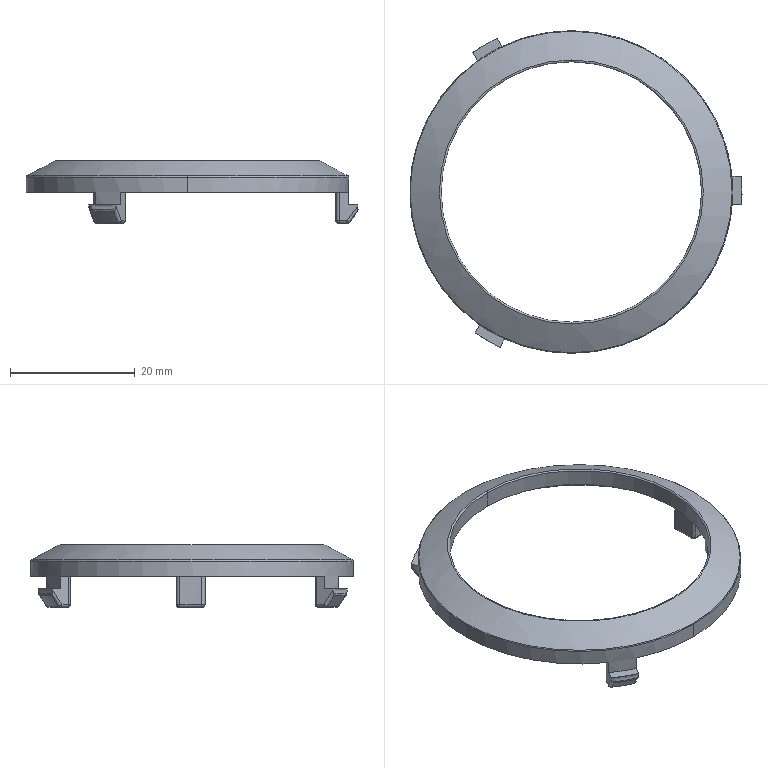Part | SolidWorks | features BaseBody 1 | 1 solid | 90 faces | box 53.3 x 51.8 x 10.109 mm | volume 2195 mm3 | cylinder 30 | plane 18 | sphere 15 | torus 14 | spline 10 | cone 3 | commonest cylinder face diameters 1 x15 0.4 x5 47.8 x3 54.8 x3 41.8 x2 51.8 x2